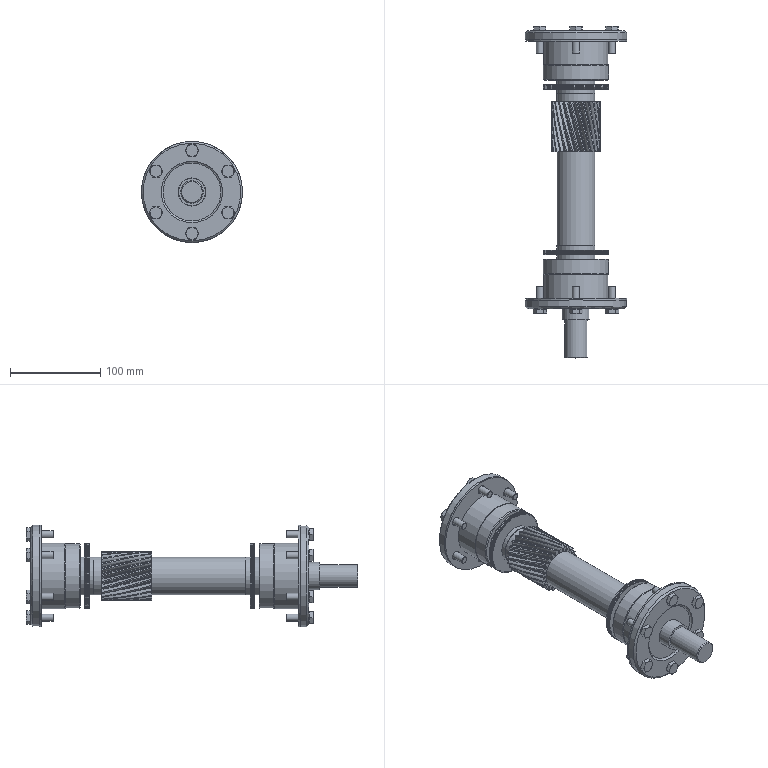Part | NX | 42 solids | 595 faces | box 112 x 366.9 x 112 mm | volume 770661 mm3 | cone 172 | plane 158 | spline 120 | cylinder 107 | torus 20 | sphere 18 | commonest cylinder face diameters 9 x24 44.92 x24 7.76 x12 11.63 x12 35 x6 42 x6